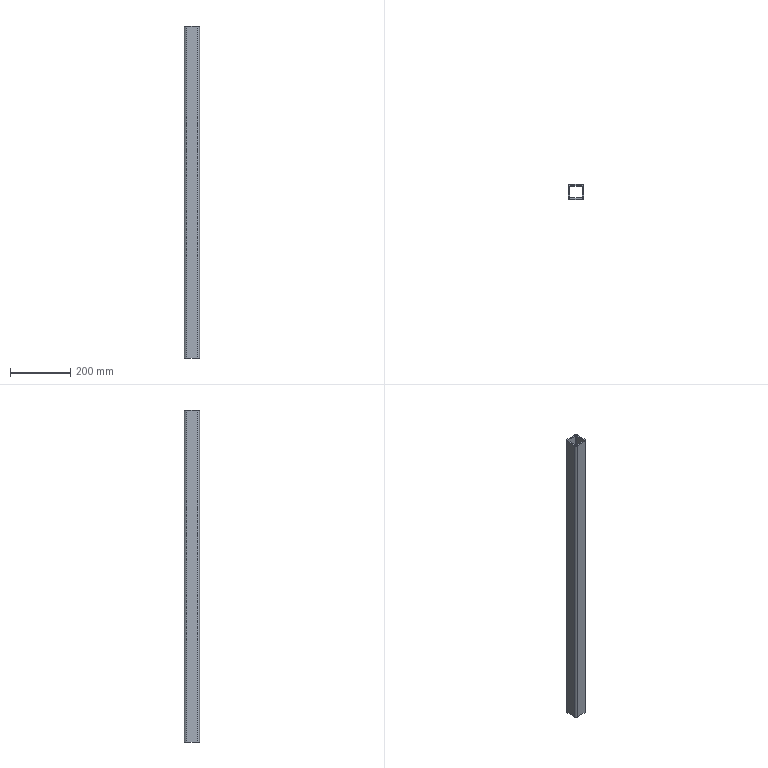Part | NX | 1 solid | 18 faces | box 50 x 50 x 1100 mm | volume 947509 mm3 | plane 10 | cylinder 8 | commonest cylinder face diameters 4 x4 14 x4
STEP:
#1=CARTESIAN_POINT('',(-895.,-18.,550.));
#2=VERTEX_POINT('',#1);
#3=CARTESIAN_POINT('',(-895.,-18.,-550.));
#4=VERTEX_POINT('',#3);
#5=CARTESIAN_POINT('',(-895.,-18.,575.));
#6=DIRECTION('',(0.,0.,-1.));
#7=VECTOR('',#6,1000.);
#8=LINE('',#5,#7);
#9=EDGE_CURVE('',#2,#4,#8,.T.);
#10=ORIENTED_EDGE('',*,*,#9,.T.);
#11=CARTESIAN_POINT('',(-895.,18.,-550.));
#12=VERTEX_POINT('',#11);
#13=CARTESIAN_POINT('',(-895.,-18.,-550.));
#14=DIRECTION('',(0.,1.,0.));
#15=VECTOR('',#14,1000.);
#16=LINE('',#13,#15);
#17=EDGE_CURVE('',#4,#12,#16,.T.);
#18=ORIENTED_EDGE('',*,*,#17,.T.);
#19=CARTESIAN_POINT('',(-895.,18.,550.));
#20=VERTEX_POINT('',#19);
#21=CARTESIAN_POINT('',(-895.,18.,575.));
#22=DIRECTION('',(0.,0.,-1.));
#23=VECTOR('',#22,1000.);
#24=LINE('',#21,#23);
#25=EDGE_CURVE('',#20,#12,#24,.T.);
#26=ORIENTED_EDGE('',*,*,#25,.F.);
#27=CARTESIAN_POINT('',(-895.,-18.,550.));
#28=DIRECTION('',(0.,-1.,0.));
#29=VECTOR('',#28,1000.);
#30=LINE('',#27,#29);
#31=EDGE_CURVE('',#20,#2,#30,.T.);
#32=ORIENTED_EDGE('',*,*,#31,.T.);
#33=EDGE_LOOP('',(#10,#18,#26,#32));
#34=FACE_BOUND('',#33,.T.);
#35=CARTESIAN_POINT('',(-895.,-18.,575.));
#36=DIRECTION('',(1.,0.,0.));
#37=DIRECTION('',(0.,1.,0.));
#38=AXIS2_PLACEMENT_3D('',#35,#36,#37);
#39=PLANE('',#38);
#40=ADVANCED_FACE('',(#34),#39,.T.);
#41=CARTESIAN_POINT('',(-893.,-20.,550.));
#42=VERTEX_POINT('',#41);
#43=CARTESIAN_POINT('',(-893.,-20.,-550.));
#44=VERTEX_POINT('',#43);
#45=CARTESIAN_POINT('',(-893.,-20.,575.));
#46=DIRECTION('',(0.,0.,-1.));
#47=VECTOR('',#46,1000.);
#48=LINE('',#45,#47);
#49=EDGE_CURVE('',#42,#44,#48,.T.);
#50=ORIENTED_EDGE('',*,*,#49,.T.);
#51=CARTESIAN_POINT('',(-893.,-18.,-550.));
#52=DIRECTION('',(0.,0.,-1.));
#53=DIRECTION('',(0.,1.,0.));
#54=AXIS2_PLACEMENT_3D('',#51,#52,#53);
#55=CIRCLE('',#54,2.);
#56=EDGE_CURVE('',#44,#4,#55,.T.);
#57=ORIENTED_EDGE('',*,*,#56,.T.);
#58=ORIENTED_EDGE('',*,*,#9,.F.);
#59=CARTESIAN_POINT('',(-893.,-18.,550.));
#60=DIRECTION('',(0.,0.,1.));
#61=DIRECTION('',(0.,-1.,0.));
#62=AXIS2_PLACEMENT_3D('',#59,#60,#61);
#63=CIRCLE('',#62,2.);
#64=EDGE_CURVE('',#2,#42,#63,.T.);
#65=ORIENTED_EDGE('',*,*,#64,.T.);
#66=EDGE_LOOP('',(#50,#57,#58,#65));
#67=FACE_BOUND('',#66,.T.);
#68=CARTESIAN_POINT('',(-893.,-18.,575.));
#69=DIRECTION('',(0.,0.,-1.));
#70=DIRECTION('',(-1.,0.,0.));
#71=AXIS2_PLACEMENT_3D('',#68,#69,#70);
#72=CYLINDRICAL_SURFACE('',#71,2.);
#73=ADVANCED_FACE('',(#67),#72,.F.);
#74=CARTESIAN_POINT('',(-857.,-20.,550.));
#75=VERTEX_POINT('',#74);
#76=CARTESIAN_POINT('',(-857.,-20.,-550.));
#77=VERTEX_POINT('',#76);
#78=CARTESIAN_POINT('',(-857.,-20.,575.));
#79=DIRECTION('',(0.,0.,-1.));
#80=VECTOR('',#79,1000.);
#81=LINE('',#78,#80);
#82=EDGE_CURVE('',#75,#77,#81,.T.);
#83=ORIENTED_EDGE('',*,*,#82,.T.);
#84=CARTESIAN_POINT('',(-893.,-20.,-550.));
#85=DIRECTION('',(-1.,0.,0.));
#86=VECTOR('',#85,1000.);
#87=LINE('',#84,#86);
#88=EDGE_CURVE('',#77,#44,#87,.T.);
#89=ORIENTED_EDGE('',*,*,#88,.T.);
#90=ORIENTED_EDGE('',*,*,#49,.F.);
#91=CARTESIAN_POINT('',(-893.,-20.,550.));
#92=DIRECTION('',(1.,0.,0.));
#93=VECTOR('',#92,1000.);
#94=LINE('',#91,#93);
#95=EDGE_CURVE('',#42,#75,#94,.T.);
#96=ORIENTED_EDGE('',*,*,#95,.T.);
#97=EDGE_LOOP('',(#83,#89,#90,#96));
#98=FACE_BOUND('',#97,.T.);
#99=CARTESIAN_POINT('',(-893.,-20.,575.));
#100=DIRECTION('',(0.,1.,0.));
#101=DIRECTION('',(-1.,0.,0.));
#102=AXIS2_PLACEMENT_3D('',#99,#100,#101);
#103=PLANE('',#102);
#104=ADVANCED_FACE('',(#98),#103,.T.);
#105=CARTESIAN_POINT('',(-855.,-18.,550.));
#106=VERTEX_POINT('',#105);
#107=CARTESIAN_POINT('',(-855.,-18.,-550.));
#108=VERTEX_POINT('',#107);
#109=CARTESIAN_POINT('',(-855.,-18.,575.));
#110=DIRECTION('',(0.,0.,-1.));
#111=VECTOR('',#110,1000.);
#112=LINE('',#109,#111);
#113=EDGE_CURVE('',#106,#108,#112,.T.);
#114=ORIENTED_EDGE('',*,*,#113,.T.);
#115=CARTESIAN_POINT('',(-857.,-18.,-550.));
#116=DIRECTION('',(0.,0.,-1.));
#117=DIRECTION('',(0.,1.,0.));
#118=AXIS2_PLACEMENT_3D('',#115,#116,#117);
#119=CIRCLE('',#118,2.);
#120=EDGE_CURVE('',#108,#77,#119,.T.);
#121=ORIENTED_EDGE('',*,*,#120,.T.);
#122=ORIENTED_EDGE('',*,*,#82,.F.);
#123=CARTESIAN_POINT('',(-857.,-18.,550.));
#124=DIRECTION('',(0.,0.,1.));
#125=DIRECTION('',(0.,-1.,0.));
#126=AXIS2_PLACEMENT_3D('',#123,#124,#125);
#127=CIRCLE('',#126,2.);
#128=EDGE_CURVE('',#75,#106,#127,.T.);
#129=ORIENTED_EDGE('',*,*,#128,.T.);
#130=EDGE_LOOP('',(#114,#121,#122,#129));
#131=FACE_BOUND('',#130,.T.);
#132=CARTESIAN_POINT('',(-857.,-18.,575.));
#133=DIRECTION('',(0.,0.,-1.));
#134=DIRECTION('',(-1.,0.,0.));
#135=AXIS2_PLACEMENT_3D('',#132,#133,#134);
#136=CYLINDRICAL_SURFACE('',#135,2.);
#137=ADVANCED_FACE('',(#131),#136,.F.);
#138=CARTESIAN_POINT('',(-855.,18.,550.));
#139=VERTEX_POINT('',#138);
#140=CARTESIAN_POINT('',(-855.,18.,-550.));
#141=VERTEX_POINT('',#140);
#142=CARTESIAN_POINT('',(-855.,18.,575.));
#143=DIRECTION('',(0.,0.,-1.));
#144=VECTOR('',#143,1000.);
#145=LINE('',#142,#144);
#146=EDGE_CURVE('',#139,#141,#145,.T.);
#147=ORIENTED_EDGE('',*,*,#146,.T.);
#148=CARTESIAN_POINT('',(-855.,18.,-550.));
#149=DIRECTION('',(0.,-1.,0.));
#150=VECTOR('',#149,1000.);
#151=LINE('',#148,#150);
#152=EDGE_CURVE('',#141,#108,#151,.T.);
#153=ORIENTED_EDGE('',*,*,#152,.T.);
#154=ORIENTED_EDGE('',*,*,#113,.F.);
#155=CARTESIAN_POINT('',(-855.,18.,550.));
#156=DIRECTION('',(0.,1.,0.));
#157=VECTOR('',#156,1000.);
#158=LINE('',#155,#157);
#159=EDGE_CURVE('',#106,#139,#158,.T.);
#160=ORIENTED_EDGE('',*,*,#159,.T.);
#161=EDGE_LOOP('',(#147,#153,#154,#160));
#162=FACE_BOUND('',#161,.T.);
#163=CARTESIAN_POINT('',(-855.,18.,575.));
#164=DIRECTION('',(-1.,0.,0.));
#165=DIRECTION('',(0.,-1.,0.));
#166=AXIS2_PLACEMENT_3D('',#163,#164,#165);
#167=PLANE('',#166);
#168=ADVANCED_FACE('',(#162),#167,.T.);
#169=CARTESIAN_POINT('',(-857.,20.,550.));
#170=VERTEX_POINT('',#169);
#171=CARTESIAN_POINT('',(-857.,20.,-550.));
#172=VERTEX_POINT('',#171);
#173=CARTESIAN_POINT('',(-857.,20.,575.));
#174=DIRECTION('',(0.,0.,-1.));
#175=VECTOR('',#174,1000.);
#176=LINE('',#173,#175);
#177=EDGE_CURVE('',#170,#172,#176,.T.);
#178=ORIENTED_EDGE('',*,*,#177,.T.);
#179=CARTESIAN_POINT('',(-857.,18.,-550.));
#180=DIRECTION('',(0.,0.,-1.));
#181=DIRECTION('',(0.,1.,0.));
#182=AXIS2_PLACEMENT_3D('',#179,#180,#181);
#183=CIRCLE('',#182,2.);
#184=EDGE_CURVE('',#172,#141,#183,.T.);
#185=ORIENTED_EDGE('',*,*,#184,.T.);
#186=ORIENTED_EDGE('',*,*,#146,.F.);
#187=CARTESIAN_POINT('',(-857.,18.,550.));
#188=DIRECTION('',(0.,0.,1.));
#189=DIRECTION('',(0.,-1.,0.));
#190=AXIS2_PLACEMENT_3D('',#187,#188,#189);
#191=CIRCLE('',#190,2.);
#192=EDGE_CURVE('',#139,#170,#191,.T.);
#193=ORIENTED_EDGE('',*,*,#192,.T.);
#194=EDGE_LOOP('',(#178,#185,#186,#193));
#195=FACE_BOUND('',#194,.T.);
#196=CARTESIAN_POINT('',(-857.,18.,575.));
#197=DIRECTION('',(0.,0.,-1.));
#198=DIRECTION('',(-1.,0.,0.));
#199=AXIS2_PLACEMENT_3D('',#196,#197,#198);
#200=CYLINDRICAL_SURFACE('',#199,2.);
#201=ADVANCED_FACE('',(#195),#200,.F.);
#202=CARTESIAN_POINT('',(-893.,20.,550.));
#203=VERTEX_POINT('',#202);
#204=CARTESIAN_POINT('',(-893.,20.,-550.));
#205=VERTEX_POINT('',#204);
#206=CARTESIAN_POINT('',(-893.,20.,575.));
#207=DIRECTION('',(0.,0.,-1.));
#208=VECTOR('',#207,1000.);
#209=LINE('',#206,#208);
#210=EDGE_CURVE('',#203,#205,#209,.T.);
#211=ORIENTED_EDGE('',*,*,#210,.T.);
#212=CARTESIAN_POINT('',(-857.,20.,-550.));
#213=DIRECTION('',(1.,0.,0.));
#214=VECTOR('',#213,1000.);
#215=LINE('',#212,#214);
#216=EDGE_CURVE('',#205,#172,#215,.T.);
#217=ORIENTED_EDGE('',*,*,#216,.T.);
#218=ORIENTED_EDGE('',*,*,#177,.F.);
#219=CARTESIAN_POINT('',(-857.,20.,550.));
#220=DIRECTION('',(-1.,0.,0.));
#221=VECTOR('',#220,1000.);
#222=LINE('',#219,#221);
#223=EDGE_CURVE('',#170,#203,#222,.T.);
#224=ORIENTED_EDGE('',*,*,#223,.T.);
#225=EDGE_LOOP('',(#211,#217,#218,#224));
#226=FACE_BOUND('',#225,.T.);
#227=CARTESIAN_POINT('',(-857.,20.,575.));
#228=DIRECTION('',(0.,-1.,0.));
#229=DIRECTION('',(1.,0.,0.));
#230=AXIS2_PLACEMENT_3D('',#227,#228,#229);
#231=PLANE('',#230);
#232=ADVANCED_FACE('',(#226),#231,.T.);
#233=ORIENTED_EDGE('',*,*,#25,.T.);
#234=CARTESIAN_POINT('',(-893.,18.,-550.));
#235=DIRECTION('',(0.,0.,-1.));
#236=DIRECTION('',(0.,1.,0.));
#237=AXIS2_PLACEMENT_3D('',#234,#235,#236);
#238=CIRCLE('',#237,2.);
#239=EDGE_CURVE('',#12,#205,#238,.T.);
#240=ORIENTED_EDGE('',*,*,#239,.T.);
#241=ORIENTED_EDGE('',*,*,#210,.F.);
#242=CARTESIAN_POINT('',(-893.,18.,550.));
#243=DIRECTION('',(0.,0.,1.));
#244=DIRECTION('',(0.,-1.,0.));
#245=AXIS2_PLACEMENT_3D('',#242,#243,#244);
#246=CIRCLE('',#245,2.);
#247=EDGE_CURVE('',#203,#20,#246,.T.);
#248=ORIENTED_EDGE('',*,*,#247,.T.);
#249=EDGE_LOOP('',(#233,#240,#241,#248));
#250=FACE_BOUND('',#249,.T.);
#251=CARTESIAN_POINT('',(-893.,18.,575.));
#252=DIRECTION('',(0.,0.,-1.));
#253=DIRECTION('',(-1.,0.,0.));
#254=AXIS2_PLACEMENT_3D('',#251,#252,#253);
#255=CYLINDRICAL_SURFACE('',#254,2.);
#256=ADVANCED_FACE('',(#250),#255,.F.);
#257=CARTESIAN_POINT('',(-850.,18.,-550.));
#258=VERTEX_POINT('',#257);
#259=CARTESIAN_POINT('',(-850.,-18.,-550.));
#260=VERTEX_POINT('',#259);
#261=CARTESIAN_POINT('',(-850.,18.,-550.));
#262=DIRECTION('',(0.,-1.,0.));
#263=VECTOR('',#262,1000.);
#264=LINE('',#261,#263);
#265=EDGE_CURVE('',#258,#260,#264,.T.);
#266=ORIENTED_EDGE('',*,*,#265,.F.);
#267=CARTESIAN_POINT('',(-850.,18.,550.));
#268=VERTEX_POINT('',#267);
#269=CARTESIAN_POINT('',(-850.,18.,575.));
#270=DIRECTION('',(0.,0.,-1.));
#271=VECTOR('',#270,1000.);
#272=LINE('',#269,#271);
#273=EDGE_CURVE('',#268,#258,#272,.T.);
#274=ORIENTED_EDGE('',*,*,#273,.F.);
#275=CARTESIAN_POINT('',(-850.,-18.,550.));
#276=VERTEX_POINT('',#275);
#277=CARTESIAN_POINT('',(-850.,18.,550.));
#278=DIRECTION('',(0.,1.,0.));
#279=VECTOR('',#278,1000.);
#280=LINE('',#277,#279);
#281=EDGE_CURVE('',#276,#268,#280,.T.);
#282=ORIENTED_EDGE('',*,*,#281,.F.);
#283=CARTESIAN_POINT('',(-850.,-18.,575.));
#284=DIRECTION('',(0.,0.,-1.));
#285=VECTOR('',#284,1000.);
#286=LINE('',#283,#285);
#287=EDGE_CURVE('',#276,#260,#286,.T.);
#288=ORIENTED_EDGE('',*,*,#287,.T.);
#289=EDGE_LOOP('',(#266,#274,#282,#288));
#290=FACE_BOUND('',#289,.T.);
#291=CARTESIAN_POINT('',(-850.,18.,575.));
#292=DIRECTION('',(-1.,0.,0.));
#293=DIRECTION('',(0.,-1.,0.));
#294=AXIS2_PLACEMENT_3D('',#291,#292,#293);
#295=PLANE('',#294);
#296=ADVANCED_FACE('',(#290),#295,.F.);
#297=CARTESIAN_POINT('',(-857.,-25.,-550.));
#298=VERTEX_POINT('',#297);
#299=CARTESIAN_POINT('',(-857.,-18.,-550.));
#300=DIRECTION('',(0.,0.,-1.));
#301=DIRECTION('',(0.,1.,0.));
#302=AXIS2_PLACEMENT_3D('',#299,#300,#301);
#303=CIRCLE('',#302,7.);
#304=EDGE_CURVE('',#260,#298,#303,.T.);
#305=ORIENTED_EDGE('',*,*,#304,.F.);
#306=ORIENTED_EDGE('',*,*,#287,.F.);
#307=CARTESIAN_POINT('',(-857.,-25.,550.));
#308=VERTEX_POINT('',#307);
#309=CARTESIAN_POINT('',(-857.,-18.,550.));
#310=DIRECTION('',(0.,0.,1.));
#311=DIRECTION('',(0.,-1.,0.));
#312=AXIS2_PLACEMENT_3D('',#309,#310,#311);
#313=CIRCLE('',#312,7.);
#314=EDGE_CURVE('',#308,#276,#313,.T.);
#315=ORIENTED_EDGE('',*,*,#314,.F.);
#316=CARTESIAN_POINT('',(-857.,-25.,575.));
#317=DIRECTION('',(0.,0.,-1.));
#318=VECTOR('',#317,1000.);
#319=LINE('',#316,#318);
#320=EDGE_CURVE('',#308,#298,#319,.T.);
#321=ORIENTED_EDGE('',*,*,#320,.T.);
#322=EDGE_LOOP('',(#305,#306,#315,#321));
#323=FACE_BOUND('',#322,.T.);
#324=CARTESIAN_POINT('',(-857.,-18.,575.));
#325=DIRECTION('',(0.,0.,-1.));
#326=DIRECTION('',(-1.,0.,0.));
#327=AXIS2_PLACEMENT_3D('',#324,#325,#326);
#328=CYLINDRICAL_SURFACE('',#327,7.);
#329=ADVANCED_FACE('',(#323),#328,.T.);
#330=CARTESIAN_POINT('',(-893.,-25.,-550.));
#331=VERTEX_POINT('',#330);
#332=CARTESIAN_POINT('',(-975.,-25.,-550.));
#333=DIRECTION('',(1.,0.,0.));
#334=VECTOR('',#333,1000.);
#335=LINE('',#332,#334);
#336=EDGE_CURVE('',#331,#298,#335,.T.);
#337=ORIENTED_EDGE('',*,*,#336,.T.);
#338=ORIENTED_EDGE('',*,*,#320,.F.);
#339=CARTESIAN_POINT('',(-893.,-25.,550.));
#340=VERTEX_POINT('',#339);
#341=CARTESIAN_POINT('',(-975.,-25.,550.));
#342=DIRECTION('',(1.,0.,0.));
#343=VECTOR('',#342,1000.);
#344=LINE('',#341,#343);
#345=EDGE_CURVE('',#340,#308,#344,.T.);
#346=ORIENTED_EDGE('',*,*,#345,.F.);
#347=CARTESIAN_POINT('',(-893.,-25.,575.));
#348=DIRECTION('',(0.,0.,-1.));
#349=VECTOR('',#348,1000.);
#350=LINE('',#347,#349);
#351=EDGE_CURVE('',#340,#331,#350,.T.);
#352=ORIENTED_EDGE('',*,*,#351,.T.);
#353=EDGE_LOOP('',(#337,#338,#346,#352));
#354=FACE_BOUND('',#353,.T.);
#355=CARTESIAN_POINT('',(-893.,-25.,575.));
#356=DIRECTION('',(0.,1.,0.));
#357=DIRECTION('',(-1.,0.,0.));
#358=AXIS2_PLACEMENT_3D('',#355,#356,#357);
#359=PLANE('',#358);
#360=ADVANCED_FACE('',(#354),#359,.F.);
#361=CARTESIAN_POINT('',(-900.,-18.,-550.));
#362=VERTEX_POINT('',#361);
#363=CARTESIAN_POINT('',(-893.,-18.,-550.));
#364=DIRECTION('',(0.,0.,-1.));
#365=DIRECTION('',(0.,1.,0.));
#366=AXIS2_PLACEMENT_3D('',#363,#364,#365);
#367=CIRCLE('',#366,7.);
#368=EDGE_CURVE('',#331,#362,#367,.T.);
#369=ORIENTED_EDGE('',*,*,#368,.F.);
#370=ORIENTED_EDGE('',*,*,#351,.F.);
#371=CARTESIAN_POINT('',(-900.,-18.,550.));
#372=VERTEX_POINT('',#371);
#373=CARTESIAN_POINT('',(-893.,-18.,550.));
#374=DIRECTION('',(0.,0.,1.));
#375=DIRECTION('',(0.,-1.,0.));
#376=AXIS2_PLACEMENT_3D('',#373,#374,#375);
#377=CIRCLE('',#376,7.);
#378=EDGE_CURVE('',#372,#340,#377,.T.);
#379=ORIENTED_EDGE('',*,*,#378,.F.);
#380=CARTESIAN_POINT('',(-900.,-18.,575.));
#381=DIRECTION('',(0.,0.,-1.));
#382=VECTOR('',#381,1000.);
#383=LINE('',#380,#382);
#384=EDGE_CURVE('',#372,#362,#383,.T.);
#385=ORIENTED_EDGE('',*,*,#384,.T.);
#386=EDGE_LOOP('',(#369,#370,#379,#385));
#387=FACE_BOUND('',#386,.T.);
#388=CARTESIAN_POINT('',(-893.,-18.,575.));
#389=DIRECTION('',(0.,0.,-1.));
#390=DIRECTION('',(-1.,0.,0.));
#391=AXIS2_PLACEMENT_3D('',#388,#389,#390);
#392=CYLINDRICAL_SURFACE('',#391,7.);
#393=ADVANCED_FACE('',(#387),#392,.T.);
#394=CARTESIAN_POINT('',(-900.,18.,-550.));
#395=VERTEX_POINT('',#394);
#396=CARTESIAN_POINT('',(-900.,-18.,-550.));
#397=DIRECTION('',(0.,1.,0.));
#398=VECTOR('',#397,1000.);
#399=LINE('',#396,#398);
#400=EDGE_CURVE('',#362,#395,#399,.T.);
#401=ORIENTED_EDGE('',*,*,#400,.F.);
#402=ORIENTED_EDGE('',*,*,#384,.F.);
#403=CARTESIAN_POINT('',(-900.,18.,550.));
#404=VERTEX_POINT('',#403);
#405=CARTESIAN_POINT('',(-900.,-18.,550.));
#406=DIRECTION('',(0.,-1.,0.));
#407=VECTOR('',#406,1000.);
#408=LINE('',#405,#407);
#409=EDGE_CURVE('',#404,#372,#408,.T.);
#410=ORIENTED_EDGE('',*,*,#409,.F.);
#411=CARTESIAN_POINT('',(-900.,18.,575.));
#412=DIRECTION('',(0.,0.,-1.));
#413=VECTOR('',#412,1000.);
#414=LINE('',#411,#413);
#415=EDGE_CURVE('',#404,#395,#414,.T.);
#416=ORIENTED_EDGE('',*,*,#415,.T.);
#417=EDGE_LOOP('',(#401,#402,#410,#416));
#418=FACE_BOUND('',#417,.T.);
#419=CARTESIAN_POINT('',(-900.,-18.,575.));
#420=DIRECTION('',(1.,0.,0.));
#421=DIRECTION('',(0.,1.,0.));
#422=AXIS2_PLACEMENT_3D('',#419,#420,#421);
#423=PLANE('',#422);
#424=ADVANCED_FACE('',(#418),#423,.F.);
#425=CARTESIAN_POINT('',(-893.,25.,-550.));
#426=VERTEX_POINT('',#425);
#427=CARTESIAN_POINT('',(-893.,18.,-550.));
#428=DIRECTION('',(0.,0.,-1.));
#429=DIRECTION('',(0.,1.,0.));
#430=AXIS2_PLACEMENT_3D('',#427,#428,#429);
#431=CIRCLE('',#430,7.);
#432=EDGE_CURVE('',#395,#426,#431,.T.);
#433=ORIENTED_EDGE('',*,*,#432,.F.);
#434=ORIENTED_EDGE('',*,*,#415,.F.);
#435=CARTESIAN_POINT('',(-893.,25.,550.));
#436=VERTEX_POINT('',#435);
#437=CARTESIAN_POINT('',(-893.,18.,550.));
#438=DIRECTION('',(0.,0.,1.));
#439=DIRECTION('',(0.,-1.,0.));
#440=AXIS2_PLACEMENT_3D('',#437,#438,#439);
#441=CIRCLE('',#440,7.);
#442=EDGE_CURVE('',#436,#404,#441,.T.);
#443=ORIENTED_EDGE('',*,*,#442,.F.);
#444=CARTESIAN_POINT('',(-893.,25.,575.));
#445=DIRECTION('',(0.,0.,-1.));
#446=VECTOR('',#445,1000.);
#447=LINE('',#444,#446);
#448=EDGE_CURVE('',#436,#426,#447,.T.);
#449=ORIENTED_EDGE('',*,*,#448,.T.);
#450=EDGE_LOOP('',(#433,#434,#443,#449));
#451=FACE_BOUND('',#450,.T.);
#452=CARTESIAN_POINT('',(-893.,18.,575.));
#453=DIRECTION('',(0.,0.,-1.));
#454=DIRECTION('',(-1.,0.,0.));
#455=AXIS2_PLACEMENT_3D('',#452,#453,#454);
#456=CYLINDRICAL_SURFACE('',#455,7.);
#457=ADVANCED_FACE('',(#451),#456,.T.);
#458=CARTESIAN_POINT('',(-857.,25.,-550.));
#459=VERTEX_POINT('',#458);
#460=CARTESIAN_POINT('',(-975.,25.,-550.));
#461=DIRECTION('',(1.,0.,0.));
#462=VECTOR('',#461,1000.);
#463=LINE('',#460,#462);
#464=EDGE_CURVE('',#426,#459,#463,.T.);
#465=ORIENTED_EDGE('',*,*,#464,.F.);
#466=ORIENTED_EDGE('',*,*,#448,.F.);
#467=CARTESIAN_POINT('',(-857.,25.,550.));
#468=VERTEX_POINT('',#467);
#469=CARTESIAN_POINT('',(-975.,25.,550.));
#470=DIRECTION('',(1.,0.,0.));
#471=VECTOR('',#470,1000.);
#472=LINE('',#469,#471);
#473=EDGE_CURVE('',#436,#468,#472,.T.);
#474=ORIENTED_EDGE('',*,*,#473,.T.);
#475=CARTESIAN_POINT('',(-857.,25.,575.));
#476=DIRECTION('',(0.,0.,-1.));
#477=VECTOR('',#476,1000.);
#478=LINE('',#475,#477);
#479=EDGE_CURVE('',#468,#459,#478,.T.);
#480=ORIENTED_EDGE('',*,*,#479,.T.);
#481=EDGE_LOOP('',(#465,#466,#474,#480));
#482=FACE_BOUND('',#481,.T.);
#483=CARTESIAN_POINT('',(-857.,25.,575.));
#484=DIRECTION('',(0.,-1.,0.));
#485=DIRECTION('',(1.,0.,0.));
#486=AXIS2_PLACEMENT_3D('',#483,#484,#485);
#487=PLANE('',#486);
#488=ADVANCED_FACE('',(#482),#487,.F.);
#489=CARTESIAN_POINT('',(-857.,18.,-550.));
#490=DIRECTION('',(0.,0.,-1.));
#491=DIRECTION('',(0.,1.,0.));
#492=AXIS2_PLACEMENT_3D('',#489,#490,#491);
#493=CIRCLE('',#492,7.);
#494=EDGE_CURVE('',#459,#258,#493,.T.);
#495=ORIENTED_EDGE('',*,*,#494,.F.);
#496=ORIENTED_EDGE('',*,*,#479,.F.);
#497=CARTESIAN_POINT('',(-857.,18.,550.));
#498=DIRECTION('',(0.,0.,1.));
#499=DIRECTION('',(0.,-1.,0.));
#500=AXIS2_PLACEMENT_3D('',#497,#498,#499);
#501=CIRCLE('',#500,7.);
#502=EDGE_CURVE('',#268,#468,#501,.T.);
#503=ORIENTED_EDGE('',*,*,#502,.F.);
#504=ORIENTED_EDGE('',*,*,#273,.T.);
#505=EDGE_LOOP('',(#495,#496,#503,#504));
#506=FACE_BOUND('',#505,.T.);
#507=CARTESIAN_POINT('',(-857.,18.,575.));
#508=DIRECTION('',(0.,0.,-1.));
#509=DIRECTION('',(-1.,0.,0.));
#510=AXIS2_PLACEMENT_3D('',#507,#508,#509);
#511=CYLINDRICAL_SURFACE('',#510,7.);
#512=ADVANCED_FACE('',(#506),#511,.T.);
#513=ORIENTED_EDGE('',*,*,#223,.F.);
#514=ORIENTED_EDGE('',*,*,#192,.F.);
#515=ORIENTED_EDGE('',*,*,#159,.F.);
#516=ORIENTED_EDGE('',*,*,#128,.F.);
#517=ORIENTED_EDGE('',*,*,#95,.F.);
#518=ORIENTED_EDGE('',*,*,#64,.F.);
#519=ORIENTED_EDGE('',*,*,#31,.F.);
#520=ORIENTED_EDGE('',*,*,#247,.F.);
#521=EDGE_LOOP('',(#513,#514,#515,#516,#517,#518,#519,#520));
#522=FACE_BOUND('',#521,.T.);
#523=ORIENTED_EDGE('',*,*,#442,.T.);
#524=ORIENTED_EDGE('',*,*,#409,.T.);
#525=ORIENTED_EDGE('',*,*,#378,.T.);
#526=ORIENTED_EDGE('',*,*,#345,.T.);
#527=ORIENTED_EDGE('',*,*,#314,.T.);
#528=ORIENTED_EDGE('',*,*,#281,.T.);
#529=ORIENTED_EDGE('',*,*,#502,.T.);
#530=ORIENTED_EDGE('',*,*,#473,.F.);
#531=EDGE_LOOP('',(#523,#524,#525,#526,#527,#528,#529,#530));
#532=FACE_BOUND('',#531,.T.);
#533=CARTESIAN_POINT('',(-975.,-18.,550.));
#534=DIRECTION('',(0.,0.,1.));
#535=DIRECTION('',(0.,-1.,0.));
#536=AXIS2_PLACEMENT_3D('',#533,#534,#535);
#537=PLANE('',#536);
#538=ADVANCED_FACE('',(#522,#532),#537,.T.);
#539=ORIENTED_EDGE('',*,*,#56,.F.);
#540=ORIENTED_EDGE('',*,*,#88,.F.);
#541=ORIENTED_EDGE('',*,*,#120,.F.);
#542=ORIENTED_EDGE('',*,*,#152,.F.);
#543=ORIENTED_EDGE('',*,*,#184,.F.);
#544=ORIENTED_EDGE('',*,*,#216,.F.);
#545=ORIENTED_EDGE('',*,*,#239,.F.);
#546=ORIENTED_EDGE('',*,*,#17,.F.);
#547=EDGE_LOOP('',(#539,#540,#541,#542,#543,#544,#545,#546));
#548=FACE_BOUND('',#547,.T.);
#549=ORIENTED_EDGE('',*,*,#368,.T.);
#550=ORIENTED_EDGE('',*,*,#400,.T.);
#551=ORIENTED_EDGE('',*,*,#432,.T.);
#552=ORIENTED_EDGE('',*,*,#464,.T.);
#553=ORIENTED_EDGE('',*,*,#494,.T.);
#554=ORIENTED_EDGE('',*,*,#265,.T.);
#555=ORIENTED_EDGE('',*,*,#304,.T.);
#556=ORIENTED_EDGE('',*,*,#336,.F.);
#557=EDGE_LOOP('',(#549,#550,#551,#552,#553,#554,#555,#556));
#558=FACE_BOUND('',#557,.T.);
#559=CARTESIAN_POINT('',(-975.,18.,-550.));
#560=DIRECTION('',(0.,0.,-1.));
#561=DIRECTION('',(0.,1.,0.));
#562=AXIS2_PLACEMENT_3D('',#559,#560,#561);
#563=PLANE('',#562);
#564=ADVANCED_FACE('',(#548,#558),#563,.T.);
#565=CLOSED_SHELL('',(#40,#73,#104,#137,#168,#201,#232,#256,#296,#329,#360,#393,#424,#457,#488,#512,#538,#564));
#566=MANIFOLD_SOLID_BREP('',#565);
#567=(LENGTH_UNIT()NAMED_UNIT(*)SI_UNIT(.MILLI.,.METRE.));
#568=UNCERTAINTY_MEASURE_WITH_UNIT(LENGTH_MEASURE(0.00001),#567,'','');
#569=(NAMED_UNIT(*)PLANE_ANGLE_UNIT()SI_UNIT($,.RADIAN.));
#570=(NAMED_UNIT(*)SI_UNIT($,.STERADIAN.)SOLID_ANGLE_UNIT());
#571=(GEOMETRIC_REPRESENTATION_CONTEXT(3)GLOBAL_UNCERTAINTY_ASSIGNED_CONTEXT((#568))GLOBAL_UNIT_ASSIGNED_CONTEXT((#567,#569,#570))REPRESENTATION_CONTEXT('',''));
#572=ADVANCED_BREP_SHAPE_REPRESENTATION('',(#566),#571);